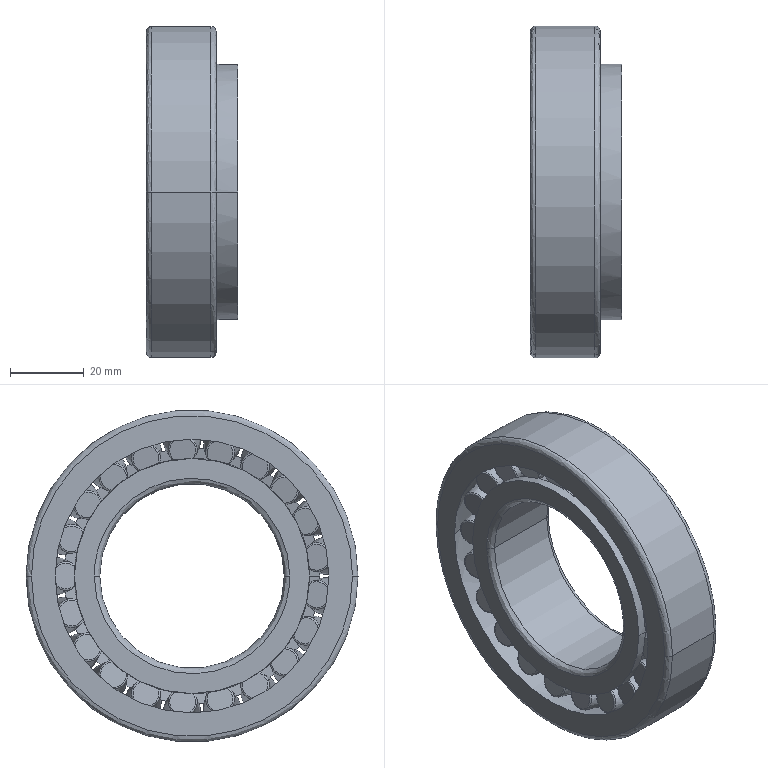Part | SolidWorks | features BaseBody 1 | 1 solid | 256 faces | box 24.75 x 90 x 90 mm | volume 73471 mm3 | spline 134 | cone 68 | plane 46 | cylinder 8 | commonest cylinder face diameters 50 x2 63.75 x2 69.336 x2 90 x2